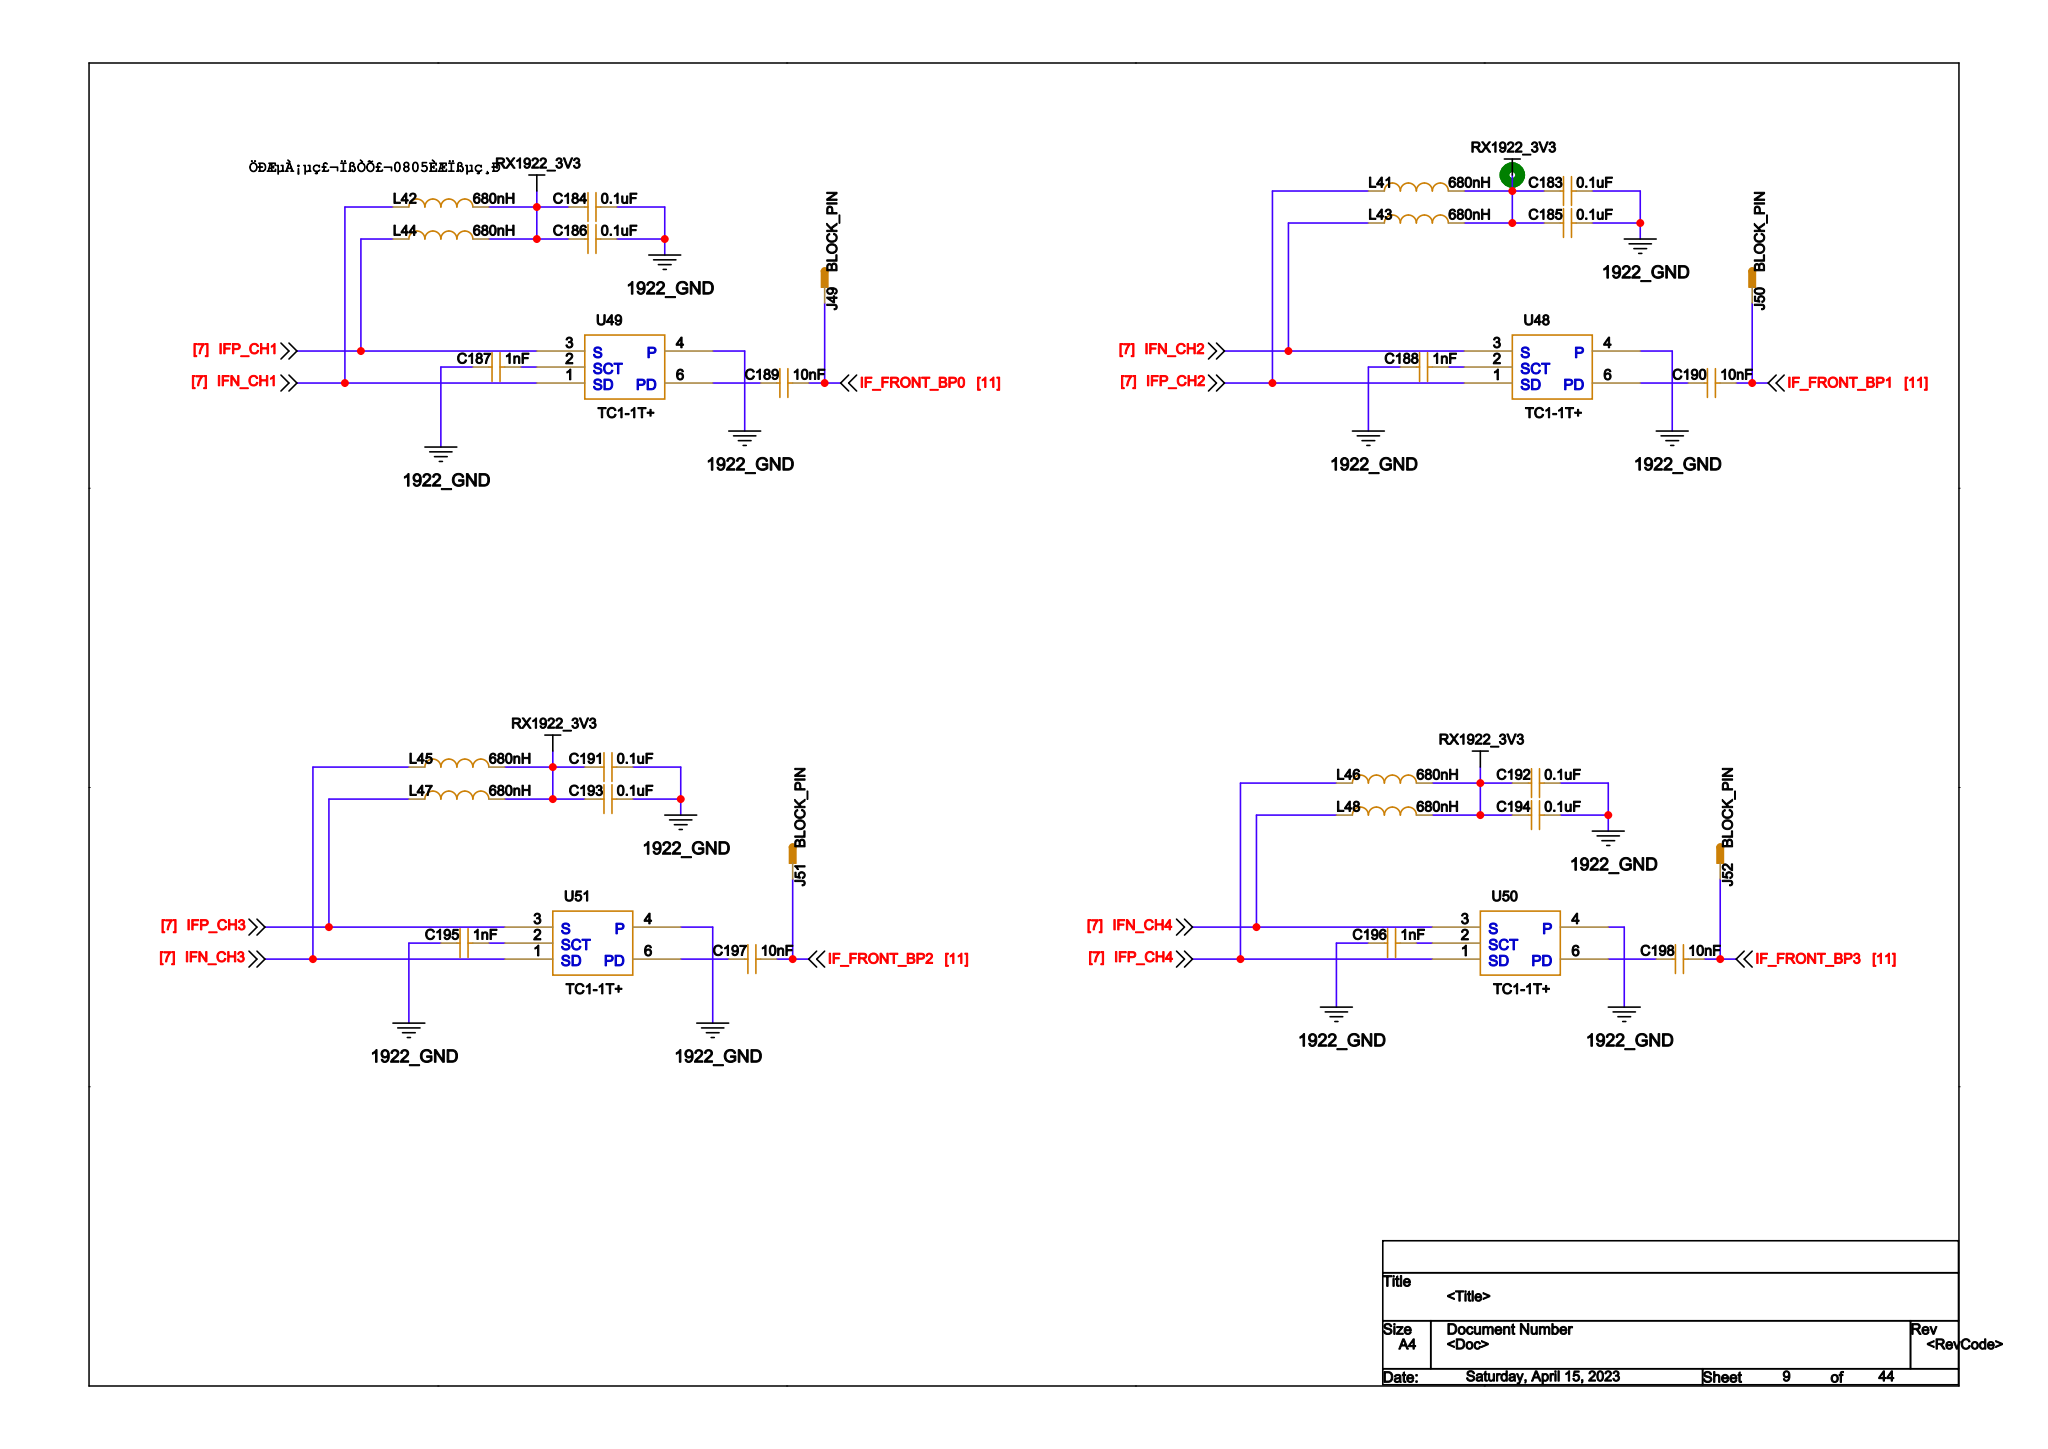Circuit board | Cadence Allegro | 1034 parts | 912 nets | one sheet of the schematic
Parts on this sheet (reference | value | footprint):
C183 | 0.1uF | C0402
C184 | 0.1uF | C0402
C185 | 0.1uF | C0402
C186 | 0.1uF | C0402
C187 | 1nF | C0402
C188 | 1nF | C0402
C189 | 10nF | C0402
C190 | 10nF | C0402
C191 | 0.1uF | C0402
C192 | 0.1uF | C0402
C193 | 0.1uF | C0402
C194 | 0.1uF | C0402
C195 | 1nF | C0402
C196 | 1nF | C0402
C197 | 10nF | C0402
C198 | 10nF | C0402
J49 | BLOCK_PIN | B_PIN_SMD
J50 | BLOCK_PIN | B_PIN_SMD
J51 | BLOCK_PIN | B_PIN_SMD
J52 | BLOCK_PIN | B_PIN_SMD
L41 | 680nH | L0805
L42 | 680nH | L0805
L43 | 680nH | L0805
L44 | 680nH | L0805
L45 | 680nH | L0805
L46 | 680nH | L0805
L47 | 680nH | L0805
L48 | 680nH | L0805
U48 | TC1-1T+ | TC1_1T_SMD
U49 | TC1-1T+ | TC1_1T_SMD
U50 | TC1-1T+ | TC1_1T_SMD
U51 | TC1-1T+ | TC1_1T_SMD
Nets of these parts (net: part-pin ...):
IF_FRONT_BP0_D2: C189-2 J49-1
IF_FRONT_BP1_D2: C190-2 J50-1
IF_FRONT_BP2_D2: C197-2 J51-1
IF_FRONT_BP3_D2: C198-2 J52-1
1922_GND: C183-2 C184-2 C185-2 C186-2 C187-1 C188-1 C191-2 C192-2 C193-2 C194-2 C195-1 C196-1 U48-4 U49-4 U50-4 U51-4
PWR1922_3V3_2: C183-1 C184-1 C185-1 C186-1 C191-1 C192-1 C193-1 C194-1 L41-2 L42-2 L43-2 L44-2 L45-2 L46-2 L47-2 L48-2
N156926_D2: C189-1 U49-6
N157763_D2: C190-1 U48-6
N158323_D2: C197-1 U51-6
N158912_D2: C198-1 U50-6
N156737_D2: C187-2 U49-2
N157727_D2: C188-2 U48-2
N158287_D2: C195-2 U51-2
N158876_D2: C196-2 U50-2
IFP_CH2_D2: L41-1 U48-1
IFN_CH1_D2: L42-1 U49-1
IFN_CH2_D2: L43-1 U48-3
IFP_CH1_D2: L44-1 U49-3
IFN_CH3_D2: L45-1 U51-1
IFP_CH4_D2: L46-1 U50-1
IFP_CH3_D2: L47-1 U51-3
IFN_CH4_D2: L48-1 U50-3